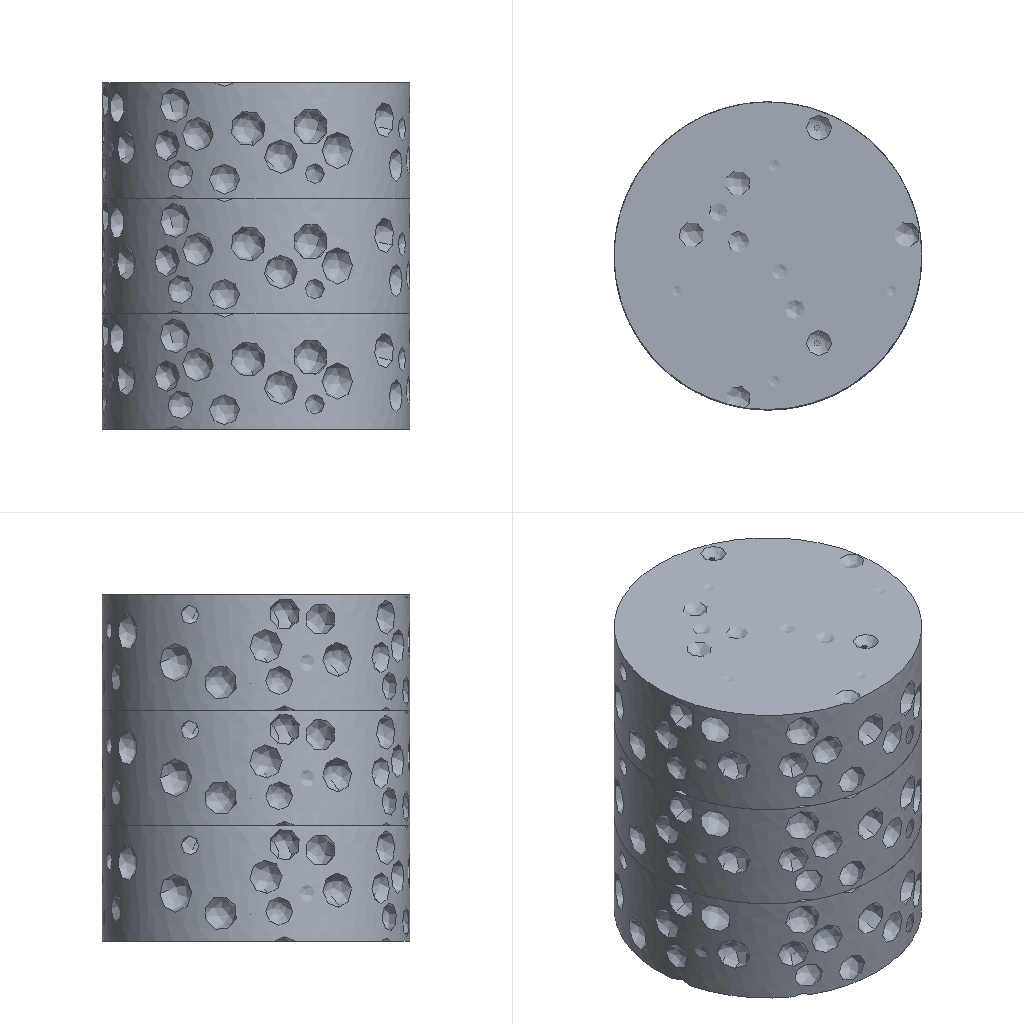Simulation study | abaqus
Set-up summary:
category,name,step,type,value,unit,region
solver,abaqus
solver,version,,,Abaqus/Standard 2020
units,not stated in the deck,,not stated
analysis,deck,,static,static
load_step,Step-1,Step-1,static,nlgeom=True
contact,interactions,,,general=0 pairs=0 ties=2
load_step,requested,,,1
mesh,nodes,,,42453
mesh,elements,,,203820
element_type,C3D4,,solid,203820
load,load commands in deck,,count,1
bc,support commands in deck,,count,1
material,MATERIAL-1,,in results
check,setup vs results,,match,"per instance, exact: element labels, types and connectivity; labels of the nodes the elements use; coordinates of those nodes at SINGLE_PRECISION in 1 of 3 instance(s)"
Abaqus input file, long lists of numbers shortened:
*Heading
** Job name: Job-1 Model name: Model-1
** Generated by: Abaqus/CAE 2020
*Preprint, echo=NO, model=NO, history=NO, contact=NO
**
** PARTS
**
*Part, name=final
*Node
      1,   12.704,  -22.061,    28.719
      2,   9.479,  -25.425,   26.872
** (14149 more lines like these left out)
*Element, type=C3D4
    1,  6753,  6754,  6755,  6756
    2,  6757,  6758,  6759,  6760
** (67938 more lines like these left out)
*Nset, nset=Set-4, generate
     1,  14151,      1
*Elset, elset=Set-4, generate
     1,  67940,      1
** Section: Section-1
*Solid Section, elset=Set-4, material=Material-1
,
*End Part
**
*Part, name=final-Copy
*Node
      1,   12.704,  -22.061,    28.719
      2,   9.479,  -25.425,   26.872
** (14149 more lines like these left out)
*Element, type=C3D4
    1,  6753,  6754,  6755,  6756
    2,  6757,  6758,  6759,  6760
** (67938 more lines like these left out)
*Nset, nset=Set-4, generate
     1,  14151,      1
*Elset, elset=Set-4, generate
     1,  67940,      1
** Section: Section-1
*Solid Section, elset=Set-4, material=Material-1
,
*End Part
**
*Part, name=final-Copy2
*Node
      1,   12.704,  -22.061,    28.719
      2,   9.479,  -25.425,   26.872
** (14149 more lines like these left out)
*Element, type=C3D4
    1,  6753,  6754,  6755,  6756
    2,  6757,  6758,  6759,  6760
** (67938 more lines like these left out)
*Nset, nset=Set-4, generate
     1,  14151,      1
*Elset, elset=Set-4, generate
     1,  67940,      1
** Section: Section-1
*Solid Section, elset=Set-4, material=Material-1
,
*End Part
**
**
** ASSEMBLY
**
*Assembly, name=Assembly
**
*Instance, name=final-1, part=final
*End Instance
**
*Instance, name=final-Copy-1, part=final-Copy
          0.,           0.,          30.
*End Instance
**
*Instance, name=final-Copy2-1, part=final-Copy2
          0.,           0.,          60.
*End Instance
**
*Nset, nset=Set-2, instance=final-1
  107,  108,  109,  110,  112,  113,  114,  115,  116,  117,  118,  119,  120,  121,  123,  124
  125,  126,  127,  128,  129,  130,  131,  132,  133,  134,  135,  771,  772,  773,  774,  775
** (69 more lines like these left out)
*Elset, elset=Set-2, instance=final-1
   918,   951,  1264,  1482,  1784,  2058,  2512,  3058,  3121,  3421,  3962,  4098,  4299,  4785,  5767,  6039
  6126,  6332,  6546,  6550,  6578,  6580,  7440,  7441,  8115,  8476,  8614,  8618,  8619,  8745,  8823,  8828
** (129 more lines like these left out)
*Elset, elset=_Surf-3_S2, internal, instance=final-Copy2-1
    33,  1019,  4689,  7835,  9380,  9417,  9477,  9662, 10046, 10536, 11556, 11899, 13203, 14609, 18303, 18622
 19193, 19210, 19281, 19308, 19323, 19416, 19599, 19906, 19932, 19940, 20150, 20338, 20411, 20507, 20796, 20813
** (3 more lines like these left out)
*Elset, elset=_Surf-3_S4, internal, instance=final-Copy2-1
    79,   188,   754,  4049,  4291,  5706,  8034,  8203,  9212,  9717, 10694, 10775, 11091, 11202, 11744, 11802
 11806, 11856, 12617, 13384, 14221, 14642, 14651, 15424, 15934, 18357, 19116, 19290, 19445, 19591, 19813, 19854
** (5 more lines like these left out)
*Elset, elset=_Surf-3_S3, internal, instance=final-Copy2-1
  1186,  1490,  1888,  2324,  2785,  2926,  3211,  3315,  3604,  6681,  6797,  7396,  8061,  8126,  8452,  8466
  8484,  8510,  8517,  8598,  8606,  8674,  8685,  8688,  8706,  8747,  8751,  8754,  8769,  8790,  8843,  8849
** (115 more lines like these left out)
*Elset, elset=_Surf-3_S1, internal, instance=final-Copy2-1
  5448,  8127, 10414, 11301, 11317, 14941, 15364, 17724, 19822, 21182, 22030, 22036, 22665, 23350, 23974, 25336
 25386, 25418, 25682, 26648, 27383, 33501, 33715, 35322, 37011, 38180, 38453, 39176, 39380, 42440, 42599, 50132
** (1 more lines like these left out)
*Surface, type=ELEMENT, name=Surf-3
_Surf-3_S2, S2
_Surf-3_S4, S4
_Surf-3_S3, S3
_Surf-3_S1, S1
*Elset, elset=_m_Surf-4_S2, internal, instance=final-1
    33,  1019,  4689,  7835,  9380,  9417,  9477,  9662, 10046, 10536, 11556, 11899, 13203, 14609, 18303, 18622
 19193, 19210, 19281, 19308, 19323, 19416, 19599, 19906, 19932, 19940, 20150, 20338, 20411, 20507, 20796, 20813
** (3 more lines like these left out)
*Elset, elset=_m_Surf-4_S4, internal, instance=final-1
    79,   188,   754,  4049,  4291,  5706,  8034,  8203,  9212,  9717, 10694, 10775, 11091, 11202, 11744, 11802
 11806, 11856, 12617, 13384, 14221, 14642, 14651, 15424, 15934, 18357, 19116, 19290, 19445, 19591, 19813, 19854
** (5 more lines like these left out)
*Elset, elset=_m_Surf-4_S3, internal, instance=final-1
  1186,  1490,  1888,  2324,  2785,  2926,  3211,  3315,  3604,  6681,  6797,  7396,  8061,  8126,  8452,  8466
  8484,  8510,  8517,  8598,  8606,  8674,  8685,  8688,  8706,  8747,  8751,  8754,  8769,  8790,  8843,  8849
** (115 more lines like these left out)
*Elset, elset=_m_Surf-4_S1, internal, instance=final-1
  5448,  8127, 10414, 11301, 11317, 14941, 15364, 17724, 19822, 21182, 22030, 22036, 22665, 23350, 23974, 25336
 25386, 25418, 25682, 26648, 27383, 33501, 33715, 35322, 37011, 38180, 38453, 39176, 39380, 42440, 42599, 50132
** (1 more lines like these left out)
*Surface, type=ELEMENT, name=m_Surf-4
_m_Surf-4_S2, S2
_m_Surf-4_S4, S4
_m_Surf-4_S3, S3
_m_Surf-4_S1, S1
*Elset, elset=_m_Surf-6_S2, internal, instance=final-Copy-1
    33,  1019,  4689,  7835,  9380,  9417,  9477,  9662, 10046, 10536, 11556, 11899, 13203, 14609, 18303, 18622
 19193, 19210, 19281, 19308, 19323, 19416, 19599, 19906, 19932, 19940, 20150, 20338, 20411, 20507, 20796, 20813
** (3 more lines like these left out)
*Elset, elset=_m_Surf-6_S4, internal, instance=final-Copy-1
    79,   188,   754,  4049,  4291,  5706,  8034,  8203,  9212,  9717, 10694, 10775, 11091, 11202, 11744, 11802
 11806, 11856, 12617, 13384, 14221, 14642, 14651, 15424, 15934, 18357, 19116, 19290, 19445, 19591, 19813, 19854
** (5 more lines like these left out)
*Elset, elset=_m_Surf-6_S3, internal, instance=final-Copy-1
  1186,  1490,  1888,  2324,  2785,  2926,  3211,  3315,  3604,  6681,  6797,  7396,  8061,  8126,  8452,  8466
  8484,  8510,  8517,  8598,  8606,  8674,  8685,  8688,  8706,  8747,  8751,  8754,  8769,  8790,  8843,  8849
** (115 more lines like these left out)
*Elset, elset=_m_Surf-6_S1, internal, instance=final-Copy-1
  5448,  8127, 10414, 11301, 11317, 14941, 15364, 17724, 19822, 21182, 22030, 22036, 22665, 23350, 23974, 25336
 25386, 25418, 25682, 26648, 27383, 33501, 33715, 35322, 37011, 38180, 38453, 39176, 39380, 42440, 42599, 50132
** (1 more lines like these left out)
*Surface, type=ELEMENT, name=m_Surf-6
_m_Surf-6_S2, S2
_m_Surf-6_S4, S4
_m_Surf-6_S3, S3
_m_Surf-6_S1, S1
*Elset, elset=_s_Surf-4_S3, internal, instance=final-Copy-1
   918,   951,  1482,  1784,  2058,  2512,  3058,  3121,  3421,  3962,  4299,  5767,  6332,  6550,  6578,  6580
  7440,  7441,  8115,  8476,  8614,  8618,  8619,  8823,  8828,  8836,  8867,  9025,  9140,  9141,  9149,  9188
** (113 more lines like these left out)
*Elset, elset=_s_Surf-4_S1, internal, instance=final-Copy-1
  1264,  6546, 12041, 12223, 17351, 20539, 20975, 23631, 23851, 24016, 24040, 24058, 24304, 25150, 26086, 26794
 27529, 28036, 28047, 28244, 28309, 28375, 29069, 29124, 29164, 29236, 29772, 30714, 32126, 34696, 39105, 40388
** (1 more lines like these left out)
*Elset, elset=_s_Surf-4_S2, internal, instance=final-Copy-1
  4098,  6126,  8745, 12213, 12683, 14206, 16997, 17311, 17586, 17975, 18068, 18131, 20503, 21877, 24038, 24228
 24248, 24259, 24745, 24883, 25015, 25094, 25329, 25340, 25466, 25775, 25935, 25964, 26350, 26649, 27285, 27778
** (5 more lines like these left out)
*Elset, elset=_s_Surf-4_S4, internal, instance=final-Copy-1
  4785,  6039,  9063,  9451,  9683, 12141, 12178, 12934, 13585, 13736, 14495, 17062, 17325, 17432, 18112, 18706
 21861, 22709, 22985, 23159, 23684, 24045, 24112, 24487, 24532, 24604, 24723, 24915, 24936, 25426, 25763, 25781
** (5 more lines like these left out)
*Surface, type=ELEMENT, name=s_Surf-4
_s_Surf-4_S3, S3
_s_Surf-4_S1, S1
_s_Surf-4_S2, S2
_s_Surf-4_S4, S4
*Elset, elset=_s_Surf-6_S3, internal, instance=final-Copy2-1
   918,   951,  1482,  1784,  2058,  2512,  3058,  3121,  3421,  3962,  4299,  5767,  6332,  6550,  6578,  6580
  7440,  7441,  8115,  8476,  8614,  8618,  8619,  8823,  8828,  8836,  8867,  9025,  9140,  9141,  9149,  9188
** (113 more lines like these left out)
*Elset, elset=_s_Surf-6_S1, internal, instance=final-Copy2-1
  1264,  6546, 12041, 12223, 17351, 20539, 20975, 23631, 23851, 24016, 24040, 24058, 24304, 25150, 26086, 26794
 27529, 28036, 28047, 28244, 28309, 28375, 29069, 29124, 29164, 29236, 29772, 30714, 32126, 34696, 39105, 40388
** (1 more lines like these left out)
*Elset, elset=_s_Surf-6_S2, internal, instance=final-Copy2-1
  4098,  6126,  8745, 12213, 12683, 14206, 16997, 17311, 17586, 17975, 18068, 18131, 20503, 21877, 24038, 24228
 24248, 24259, 24745, 24883, 25015, 25094, 25329, 25340, 25466, 25775, 25935, 25964, 26350, 26649, 27285, 27778
** (5 more lines like these left out)
*Elset, elset=_s_Surf-6_S4, internal, instance=final-Copy2-1
  4785,  6039,  9063,  9451,  9683, 12141, 12178, 12934, 13585, 13736, 14495, 17062, 17325, 17432, 18112, 18706
 21861, 22709, 22985, 23159, 23684, 24045, 24112, 24487, 24532, 24604, 24723, 24915, 24936, 25426, 25763, 25781
** (5 more lines like these left out)
*Surface, type=ELEMENT, name=s_Surf-6
_s_Surf-6_S3, S3
_s_Surf-6_S1, S1
_s_Surf-6_S2, S2
_s_Surf-6_S4, S4
** Constraint: Constraint-2
*Tie, name=Constraint-2, adjust=yes
s_Surf-4, m_Surf-4
** Constraint: Constraint-3
*Tie, name=Constraint-3, adjust=yes
s_Surf-6, m_Surf-6
*End Assembly
*Amplitude, name=Amp-1
             0.,              0.,              1.,              1.
**
** MATERIALS
**
*Material, name=Material-1
*Density
 2.7e-09,
*Elastic
24968., 0.22
** ----------------------------------------------------------------
**
** STEP: Step-1
**
*Step, name=Step-1, nlgeom=YES, inc=1000
*Static, stabilize=0.0002, allsdtol=0.05, continue=NO
0.01, 1., 1e-05, 0.1
**
** BOUNDARY CONDITIONS
**
** Name: BC-1 Type: 对称/反对称/完全固定
*Boundary
Set-2, ENCASTRE
**
** LOADS
**
** Name: Load-1   Type: Pressure
*Dsload, amplitude=Amp-1
Surf-3, P, 50.
**
** OUTPUT REQUESTS
**
*Restart, write, frequency=0
**
** FIELD OUTPUT: F-Output-1
**
*Output, field
*Node Output
CF, RF, U
*Element Output, directions=YES
E, LE, MISES, MISESMAX, NE, PE, PEEQ, PEMAG, S
*Contact Output
CDISP, CSTRESS
**
** HISTORY OUTPUT: H-Output-1
**
*Output, history, variable=PRESELECT
*End Step
Results summary:
result,step,,completed,increments=15 time=1.0/1.0
result,analysis,,,static
result,last_loadstep,,,1
result,analysis steps,,count,1
result,primary field,,,U
result,reaction total,,FX,-48.056,model units
result,reaction total,,FY,7.592,model units
result,reaction total,,FZ,237258.386,model units